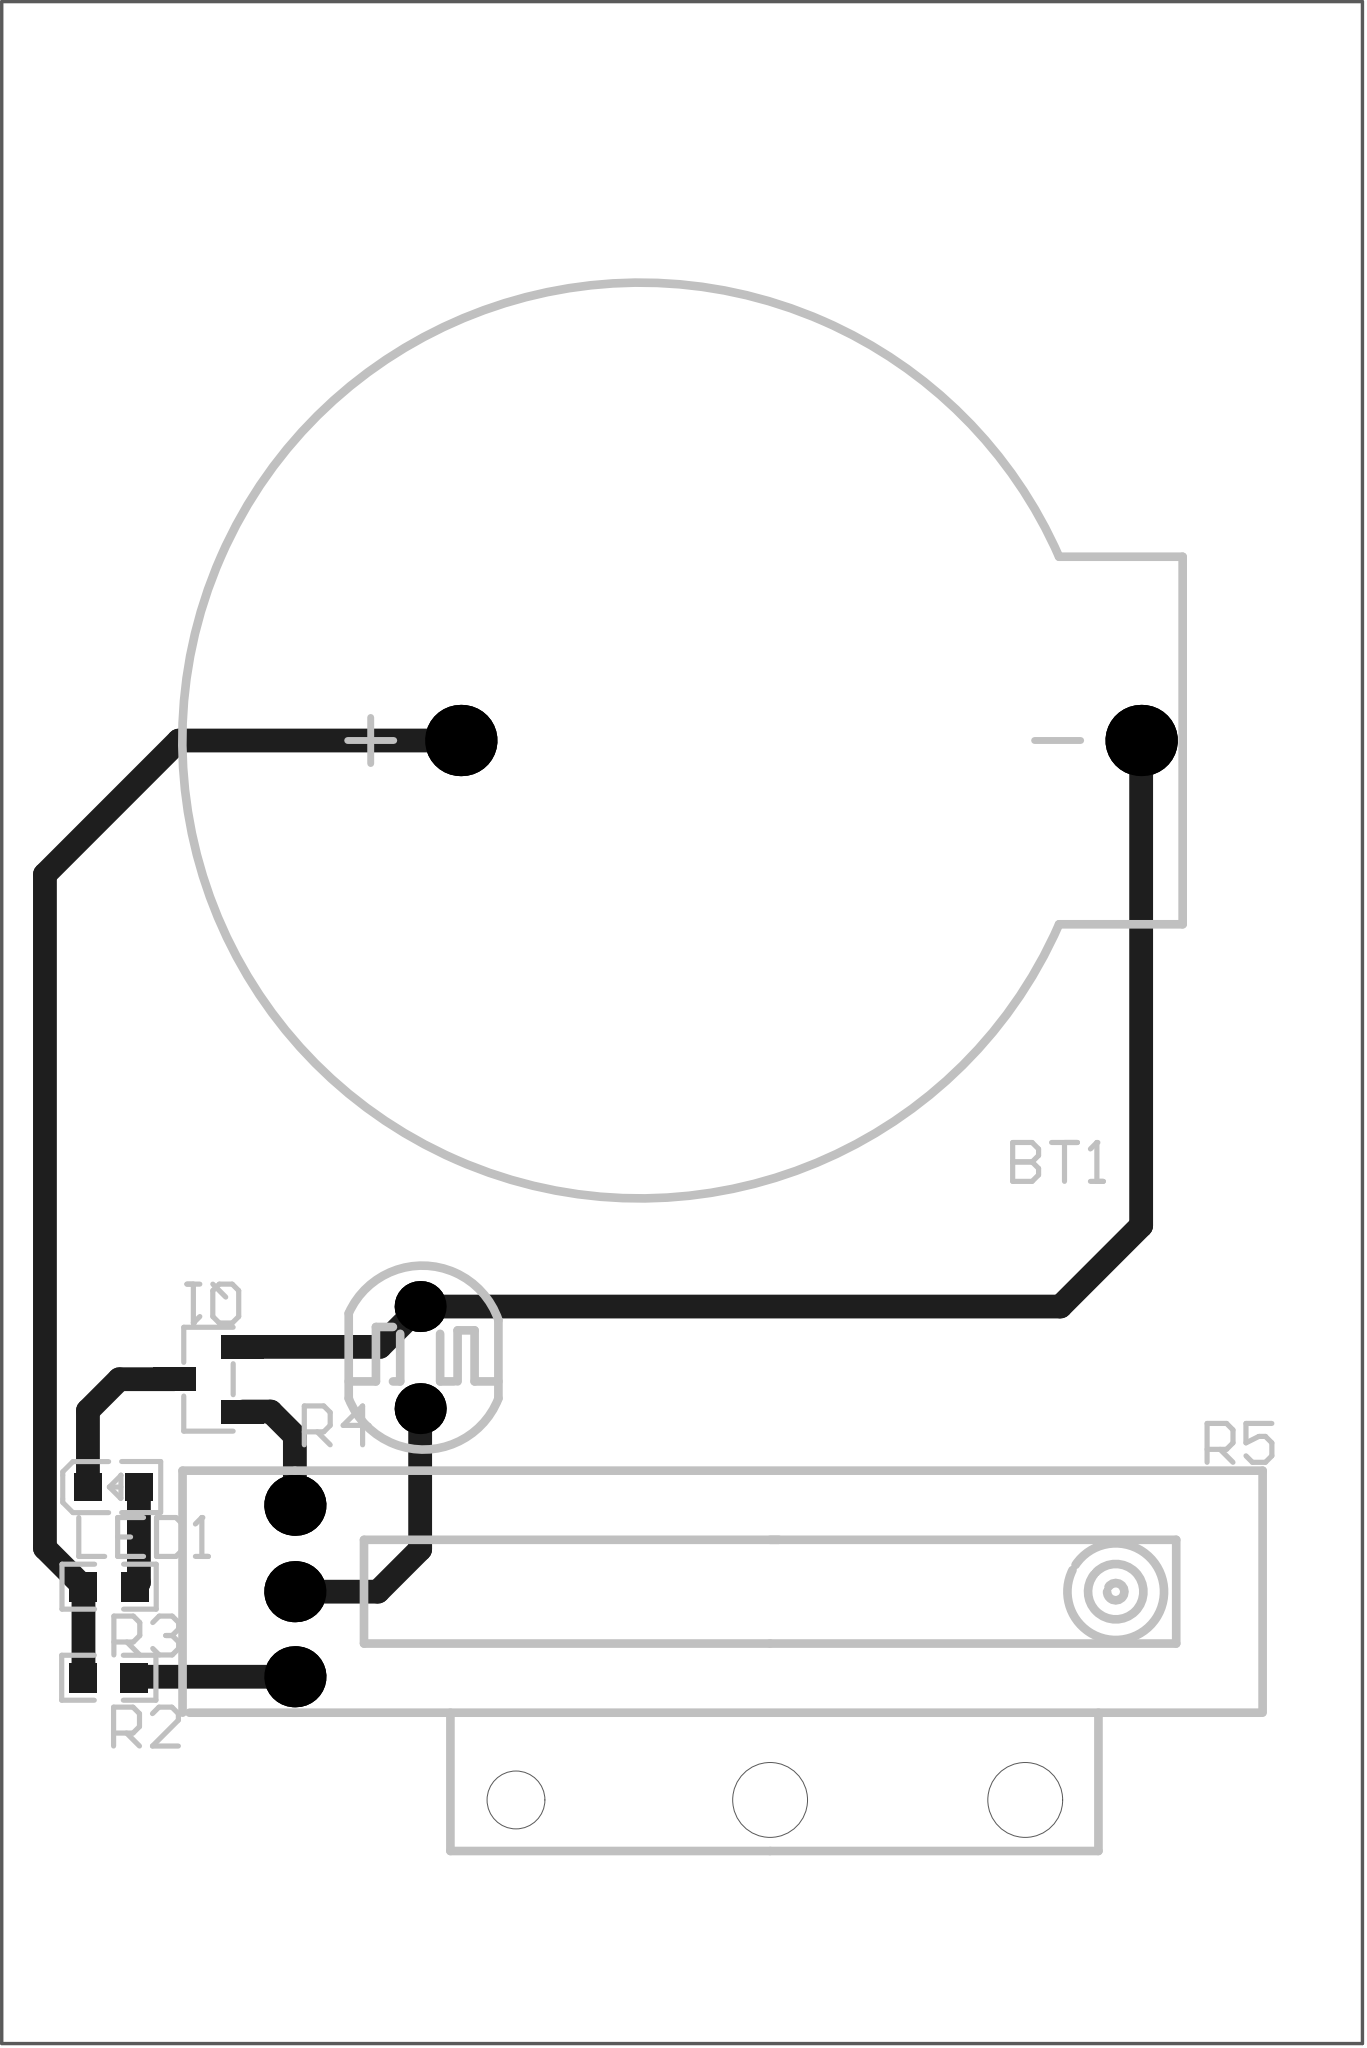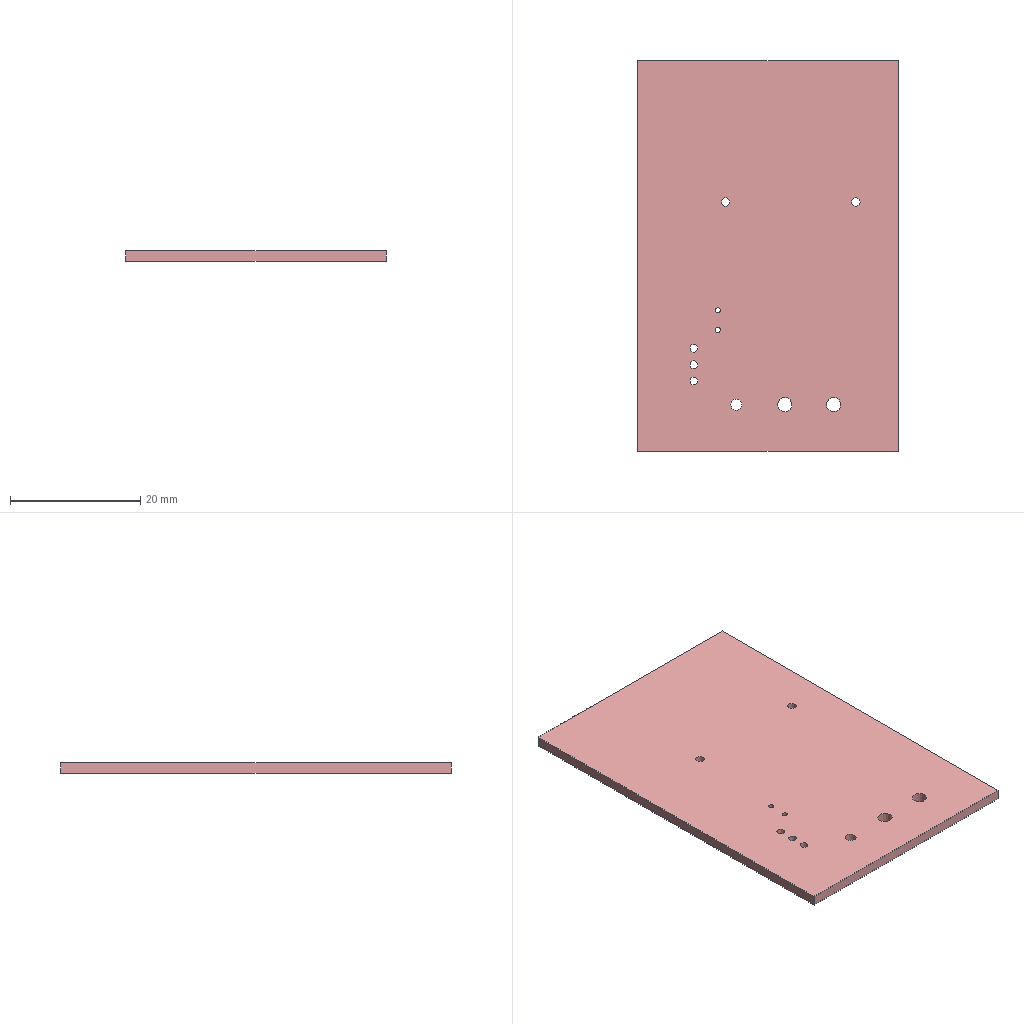Circuit board layout | Altium Designer | box 40 x 60 x 1.6 mm
Layer stack:
# Altium Designer layer stack of  (unit mm; dielectric type: 0 none, 1 core, 2 prepreg, 3 surface material)
index,name,kind,layer,copper_thickness_mm,dielectric_type,dielectric_thickness_mm,dielectric_material,dielectric_constant
0,Top Paste Mask Layer,other,,,,,,
1,Top Silkscreen Layer,other,,,,,,
2,Top Solder Mask Layer,dielectric,,,3,0.01,,3.3
3,Top Layer,copper,Top Layer,0.035,,,,
4,Dielectric1,dielectric,,,3,1.51,FR4,4.5
5,Bottom Layer,copper,Bottom Layer,0.035,,,,
6,Bottom Solder Mask Layer,dielectric,,,3,0.01,,3.3
7,Bottom Silkscreen Layer,other,,,,,,
8,Bottom Paste Mask Layer,other,,,,,,
# drill layer pairs: low layer,high layer
drill_pair,Top Layer,Bottom Layer
Part placement:
Designator,Comment,Layer,Footprint,Center-X(mm),Center-Y(mm),Rotation
BT1,79578211,TopLayer,BAT-TH_79578211,99.695,114.488,180
LED1,NCD0603Y2,TopLayer,LED0603-RD,79.484,92.546,0
Q1,SS8050,TopLayer,SOT-23-3_L2.9-W1.3-P1.90-LS2.4-BR,82.278,95.721,0
R2,10K,TopLayer,R0603,79.348,86.949,180
R3,10K,TopLayer,R0603,79.356,89.625,180
R4,GL5506(4-7K),TopLayer,RES-TH_L5.1-W4.3-P3.00-D0.5,88.501,96.356,90
R5,10kΩ,TopLayer,RES-ADJ-TH_RDC1022A05,84.817,89.498,180
Pad and via stacks:
# Altium Designer via and pad stacks of  (unit mm). Each distinct definition once, with the count of objects using it.
# via: kind,start_layer,end_layer,hole_mm,diameter_mm,mode(0 simple;1 top-mid-bottom;2 full stack),diameter_per_layer,count,example_net
# pad: kind,layer,hole_mm,hole_type(0 round;1 square;2 slot),plating,top_size,top_shape(1 round;2 rect;3 octagon;9 rounded rect),mid_size,bottom_size,mode,footprint,size_per_layer,count,example
pad,Multi-Layer,1.3,0,plated,2.1x2.1,1,2.1x2.1,2.1x2.1,0,BAT-TH_79578211,,2,BT1.1
pad,Multi-Layer,0.8,0,plated,1.5x1.5,1,1.5x1.5,1.5x1.5,0,RES-TH_L5.1-W4.3-P3.00-D0.5,,2,R4.2
pad,Multi-Layer,1.2,0,plated,1.8x1.8,1,1.8x1.8,1.8x1.8,0,RES-ADJ-TH_RDC1022A05,,3,R5.3
pad,Top Layer,0,0,plated,0.8x0.8,2,0.8x0.8,0.8x0.8,0,LED0603-RD,,2,LED1.2
pad,Top Layer,0,0,plated,1.25x0.7,2,1.25x0.7,1.25x0.7,0,SOT-23-3_L2.9-W1.3-P1.90-LS2.4-BR,,3,Q1.1
pad,Top Layer,0,0,plated,0.8065x0.864,2,0.8065x0.864,0.8065x0.864,0,R0603,,4,R2.2